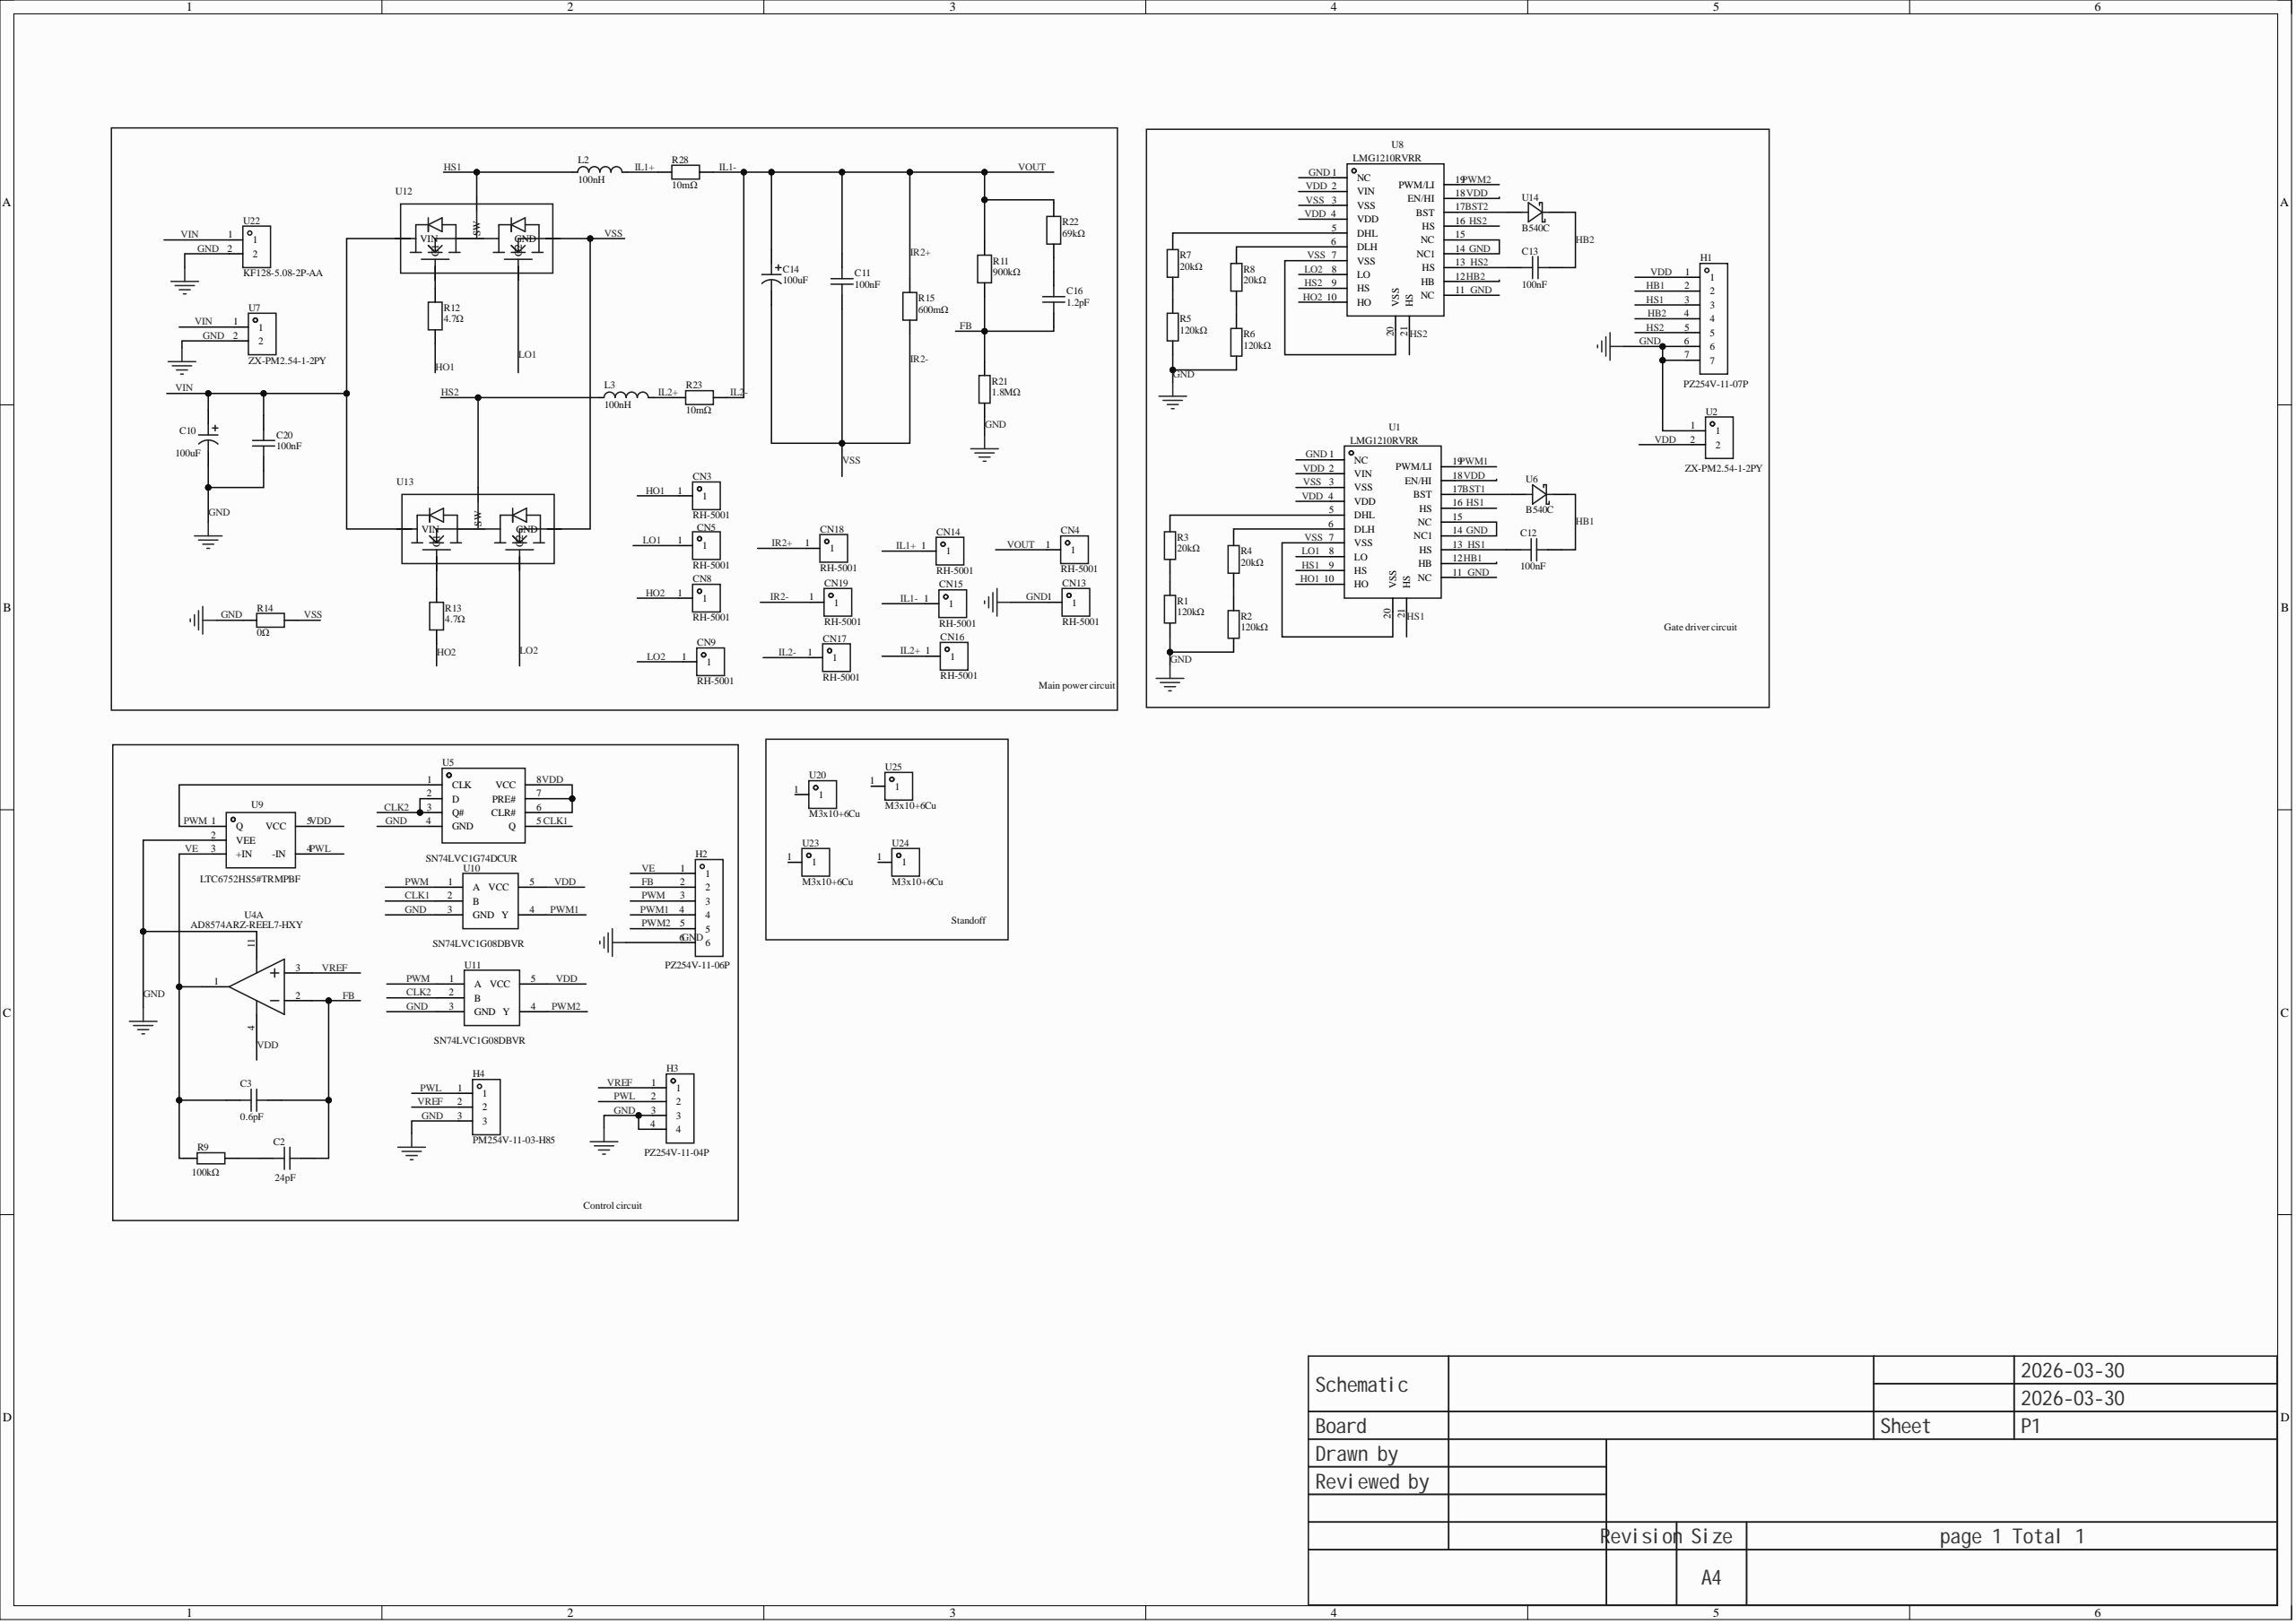Circuit board | Altium Designer | 63 parts | 38 nets
Bill of materials:
Comment,Description,Designator,Footprint,LibRef,Quantity
"24pF","Capacitance: 24pF; tolerance: ±1%; rated voltage: 50V; temperature coefficient: NP0;","C2","C0805","CC0805FRNPO9BN240","1"
"0.6pF","Capacitance: 0.6pF; rated voltage: 50V; temperature coefficient: C0G;","C3","C0603","GRM1885C1HR60WA01D","1"
"100uF","Capacitance: 100uF; tolerance: ±20%; rated voltage: 50V; ripple current: 140mA@120Hz;","C10","CAP-SMD_BD6.3-L6.6-W6.6-LS7.3-FD-H7.7","JVJ50V100M6x8","1"
"100nF","Capacitance: 100nF; tolerance: ±10%; rated voltage: 50V; temperature coefficient: X7R;","C11, C12, C13, C20","CAP-SMD_L2.0-W1.25","FCC0805B104K500DT","4"
"100uF","Capacitance: 100uF; tolerance: ±20%; rated voltage: 35V; ripple current: 2.9A@100kHz; equivalent series resistance (ESR): 30mΩ@100kHz; type: polymer;","C14","CAP-SMD_BD6.3-L6.6-W6.6-RD","MA35V100M6X8","1"
"1.2pF","Capacitance: 1.2pF; rated voltage: 250V; temperature coefficient: -;","C16","C0805","MCA08HQ1R2C251T7","1"
"RH-5001","Test pin, high-temperature nylon / phosphor bronze silver-plated, 5001 test point, 100x80mm","CN3, CN4, CN5, CN8, CN9, CN13, CN14, CN15, CN16, CN17, CN18, CN19","TEST-TH_BD2.54-P1.4_BLACK","RH-5001","12"
"PZ254V-11-07P","","H1","HDR-TH_7P-P2.54-V-M","PZ254V-11-07P","1"
"PZ254V-11-06P","","H2","HDR-TH_6P-P2.54-V-M","PZ254V-11-06P","1"
"PZ254V-11-04P","","H3","HDR-TH_4P-P2.54-V-M","PZ254V-11-04P","1"
"PM254V-11-03-H85","","H4","HDR-TH_3P-P2.54-V-F","PM254V-11-03-H85","1"
"100nH","Inductance: 100nH; tolerance: ±5%; rated current: 400mA; DC resistance (DCR): 460mΩ;","L2, L3","IND-SMD_L2.3-W1.8","AHW2012C-R10JTF","2"
"120kΩ","Resistor type: thick film resistor; resistance: 120kΩ; tolerance: ±1%; power: 125mW; working voltage: 150V; temperature coefficient: ±100ppm/?;","R1, R2, R5, R6","R0805","0805W8F1203T5E","4"
"20kΩ","Resistor type: thick film resistor; resistance: 20kΩ; tolerance: ±1%; power: 125mW; maximum working voltage: 150V; temperature coefficient: ±100ppm/?;","R3, R4, R7, R8","R0805","0805W8F2002T5E","4"
"100kΩ","Resistor type: thick film resistor; resistance: 100kΩ; tolerance: ±1%; power: 125mW; working voltage: 150V; temperature coefficient: ±100ppm/?;","R9","R0805","0805W8F1003T5E","1"
"900kΩ","Resistor type: thin film resistor; resistance: 900kΩ; tolerance: ±0.1%; power: 250mW; temperature coefficient: ±50ppm/?;","R11","R1206","RT1206BRE07900KL","1"
"4.7Ω","Resistor type: thick film resistor; resistance: 4.7Ω; tolerance: ±5%; power: 125mW; working voltage: 150V; temperature coefficient: ±200ppm/?;","R12, R13","R0805","FRC0805J4R7 TS","2"
"0Ω","Resistor type: sampling resistor; alloy resistor; resistance: 0Ω; tolerance: ±1%; power: 1W; mounting: SMD;","R14","R1206","RE1206F1R000","1"
"600mΩ","Resistor type: thick film resistor; resistance: 600mΩ; tolerance: ±1%; power: 250mW; working voltage: 500V; temperature coefficient: ±200ppm/?;","R15","R1206","FRL1206FR600TS","1"
"1.8MΩ","Resistor type: thick film resistor; resistance: 1.8MΩ; tolerance: ±1%; power: 125mW; working voltage: 150V; temperature coefficient: ±100ppm/?;","R21","R0805","0805W8F1804T5E","1"
"69kΩ","Resistor type: thin film resistor; resistance: 69kΩ; tolerance: ±0.1%; power: 100mW; temperature coefficient: ±25ppm/?;","R22","R0603","RT0603BRD0769KL","1"
"10mΩ","Resistor type: alloy resistor; resistance: 10mΩ; tolerance: ±1%; power: 750mW; temperature coefficient: ±50ppm/?; mounting: SMD;","R23, R28","R0805","RE0805FBR010","2"
"LMG1210RVRR","Driver configuration: half-bridge; load type: MOSFET; driver channels: 2; sink current (IOL): 3A; source current (IOH): 1.5A; working voltage: 6V~18V; rise time (tr): 500ps; fall time (tf): 2.3ns;","U1, U8","WQFN-19_L4.0-W3.0-P0.50-BL-EP_LMG1210RVRR","LMG1210RVRR","2"
"ZX-PM2.54-1-2PY","","U2, U7","HDR-TH_2P-P2.54-V-F","ZX-PM2.54-1-2PY","2"
"AD8574ARZ-REEL7-HXY","Amplifier count: quad; gain-bandwidth product (GBP): 1.5MHz; input bias current (Ib): 70pA; input offset voltage (Vos): 2uV; slew rate (SR): 1.2V/us; rail-to-rail: rail-to-rail input, rail-to-rail output;","U4","SOP-14_L8.7-W3.9-P1.27-LS6.0-BL","AD8574ARZ-REEL7-HXY","1"
"SN74LVC1G74DCUR","Type: D-type; working voltage: 1.65V~5.5V; clock frequency (fc): 200MHz; number of elements: 1; bits per element: 1; propagation delay (tpd): 6.4ns@5V,50pF; quiescent current (Iq): 10uA;","U5","SSOP-8_L2.0-W2.3-P0.50-LS3.1-BR","SN74LVC1G74DCUR","1"
"B540C","Diode configuration: single; forward voltage (Vf): 550mV@5A; DC reverse voltage (Vr): 40V; rectifier current: 5A;","U6, U14","SMC_L6.9-W5.9-LS7.9-RD","B540C_C6807783","2"
"LTC6752HS5#TRMPBF","Comparator count: single; input offset voltage (Vos): 1.2mV; input bias current (Ib): 1.35uA; rail-to-rail: rail-to-rail input;","U9","SOT-23-5_L3.0-W1.7-P0.95-LS2.8-BL","LTC6752HS5#TRMPBF","1"
"SN74LVC1G08DBVR","Logic type: AND gate; channels: 1; working voltage: 1.65V~5.5V; quiescent current (Iq): 10uA; propagation delay (tpd): 4ns@5V,50pF;","U10, U11","SOT-23-5_L3.0-W1.7-P0.95-LS2.8-BR","SN74LVC1G08DBVR","2"
"","","U12, U13","2111","EPC2111","2"
"M3x10+6Cu","M3x10+6","U20, U23, U24, U25","SMD_L4.7-W4.7-D3.0","M3x10+6Cu","4"
"KF128-5.08-2P-AA","","U22","CONN-TH_P5.08_KF128-5.08-2P","KF128-5.08-2P-AA","1"
Netlist (Protel format):
[
C2
C0805
24pF



]
[
C3
C0603
0.6pF



]
[
C10
CAP-SMD_BD6.3-L6.6-W6.6-LS7.3-FD-H7.7
100uF



]
[
C11
CAP-SMD_L2.0-W1.25
100nF



]
[
C12
CAP-SMD_L2.0-W1.25
100nF



]
[
C13
CAP-SMD_L2.0-W1.25
100nF



]
[
C14
CAP-SMD_BD6.3-L6.6-W6.6-RD
100uF



]
[
C16
C0805
1.2pF



]
[
C20
CAP-SMD_L2.0-W1.25
100nF



]
[
CN3
TEST-TH_BD2.54-P1.4_BLACK
RH-5001



]
[
CN4
TEST-TH_BD2.54-P1.4_BLACK
RH-5001



]
[
CN5
TEST-TH_BD2.54-P1.4_BLACK
RH-5001



]
[
CN8
TEST-TH_BD2.54-P1.4_BLACK
RH-5001



]
[
CN9
TEST-TH_BD2.54-P1.4_BLACK
RH-5001



]
[
CN13
TEST-TH_BD2.54-P1.4_BLACK
RH-5001



]
[
CN14
TEST-TH_BD2.54-P1.4_BLACK
RH-5001



]
[
CN15
TEST-TH_BD2.54-P1.4_BLACK
RH-5001



]
[
CN16
TEST-TH_BD2.54-P1.4_BLACK
RH-5001



]
[
CN17
TEST-TH_BD2.54-P1.4_BLACK
RH-5001



]
[
CN18
TEST-TH_BD2.54-P1.4_BLACK
RH-5001



]
[
CN19
TEST-TH_BD2.54-P1.4_BLACK
RH-5001



]
[
H1
HDR-TH_7P-P2.54-V-M
PZ254V-11-07P



]
[
H2
HDR-TH_6P-P2.54-V-M
PZ254V-11-06P



]
[
H3
HDR-TH_4P-P2.54-V-M
PZ254V-11-04P



]
[
H4
HDR-TH_3P-P2.54-V-F
PM254V-11-03-H85



]
[
L2
IND-SMD_L2.3-W1.8
100nH



]
[
L3
IND-SMD_L2.3-W1.8
100nH



]
[
R1
R0805
120kΩ



]
[
R2
R0805
120kΩ



]
[
R3
R0805
20kΩ



]
[
R4
R0805
20kΩ



]
[
R5
R0805
120kΩ



]
[
R6
R0805
120kΩ



]
[
R7
R0805
20kΩ



]
[
R8
R0805
20kΩ



]
[
R9
R0805
100kΩ



]
[
R11
R1206
900kΩ



]
[
R12
R0805
4.7Ω



]
[
R13
R0805
4.7Ω



]
[
R14
R1206
0Ω



]
[
R15
R1206
600mΩ



]
[
R21
R0805
1.8MΩ



]
[
R22
R0603
69kΩ



]
[
R23
R0805
10mΩ



]
[
R28
R0805
10mΩ



]
[
U1
WQFN-19_L4.0-W3.0-P0.50-BL-EP_LMG1210RVRR
LMG1210RVRR



]
[
U2
HDR-TH_2P-P2.54-V-F
ZX-PM2.54-1-2PY



]
[
U4
SOP-14_L8.7-W3.9-P1.27-LS6.0-BL
AD8574ARZ-REEL7-HXY



]
[
U5
SSOP-8_L2.0-W2.3-P0.50-LS3.1-BR
SN74LVC1G74DCUR



]
[
U6
SMC_L6.9-W5.9-LS7.9-RD
B540C



]
[
U7
HDR-TH_2P-P2.54-V-F
ZX-PM2.54-1-2PY



]
[
U8
WQFN-19_L4.0-W3.0-P0.50-BL-EP_LMG1210RVRR
LMG1210RVRR



]
[
U9
SOT-23-5_L3.0-W1.7-P0.95-LS2.8-BL
LTC6752HS5#TRMPBF



]
[
U10
SOT-23-5_L3.0-W1.7-P0.95-LS2.8-BR
SN74LVC1G08DBVR



]
[
U11
SOT-23-5_L3.0-W1.7-P0.95-LS2.8-BR
SN74LVC1G08DBVR



]
[
U12
2111




]
[
U13
2111




]
[
U14
SMC_L6.9-W5.9-LS7.9-RD
B540C



]
[
U20
SMD_L4.7-W4.7-D3.0
M3x10+6Cu



]
[
U22
CONN-TH_P5.08_KF128-5.08-2P
KF128-5.08-2P-AA



]
[
U23
SMD_L4.7-W4.7-D3.0
M3x10+6Cu



]
[
U24
SMD_L4.7-W4.7-D3.0
M3x10+6Cu



]
[
U25
SMD_L4.7-W4.7-D3.0
M3x10+6Cu



]
(
VREF
H3-1
H4-2
U4-3
)
(
VIN
C10-1
C20-2
U7-1
U12-2
U13-2
U22-1
)
(
VE
C3-1
H2-1
R9-1
U4-1
U9-3
)
(
VDD
H1-1
U1-2
U1-4
U1-18
U2-2
U4-4
U5-6
U5-7
U5-8
U8-2
U8-4
U8-18
U9-5
U10-5
U11-5
)
(
PWM2
H2-5
U8-19
U11-4
)
(
PWM1
H2-4
U1-19
U10-4
)
(
PWM
H2-3
U5-1
U9-1
U10-1
U11-1
)
(
PWL
H3-2
H4-1
U9-4
)
(
NetR13_2
R13-2
U13-1
)
(
NetR12_2
R12-2
U12-1
)
(
NetR8_2
R8-2
U8-6
)
(
NetR7_2
R7-2
U8-5
)
(
NetR6_2
R6-2
R8-1
)
(
NetR5_2
R5-2
R7-1
)
(
NetR4_2
R4-2
U1-6
)
(
NetR3_2
R3-2
U1-5
)
(
NetR2_2
R2-2
R4-1
)
(
NetR1_2
R1-2
R3-1
)
(
NetC16_2
C16-2
R22-1
)
(
NetC2_1
C2-1
R9-2
)
(
LO2
CN9-1
U8-8
U13-3
)
(
LO1
CN5-1
U1-8
U12-3
)
(
IR2-
C11-1
C14-2
CN19-1
R14-2
R15-1
U1-3
U1-7
U1-20
U8-3
U8-7
U8-20
U12-4
U13-4
)
(
IL2+
CN16-1
L3-2
R23-1
)
(
IL1-
C11-2
C14-1
CN4-1
CN15-1
CN17-1
CN18-1
R11-2
R15-2
R22-2
R23-2
R28-2
)
(
IL1+
CN14-1
L2-2
R28-1
)
(
HS2
C13-1
H1-5
L3-1
U8-9
U8-13
U8-16
U8-21
U13-5
)
(
HS1
C12-1
H1-3
L2-1
U1-9
U1-13
U1-16
U1-21
U12-5
)
(
HO2
CN8-1
R13-1
U8-10
)
(
HO1
CN3-1
R12-1
U1-10
)
(
HB2
C13-2
H1-4
U8-12
U14-1
)
(
HB1
C12-2
H1-2
U1-12
U6-1
)
(
GND
C10-2
C20-1
CN13-1
H1-6
H1-7
H2-6
H3-3
H3-4
H4-3
R1-1
R2-1
R5-1
R6-1
R14-1
R21-1
U1-1
U1-11
U1-14
U1-15
U2-1
U4-11
U5-4
U7-2
U8-1
U8-11
U8-14
U8-15
U9-2
U10-3
U11-3
U22-2
)
(
FB
C2-2
C3-2
C16-1
H2-2
R11-1
R21-2
U4-2
)
(
CLK2
U5-2
U5-3
U11-2
)
(
CLK1
U5-5
U10-2
)
(
BST2
U8-17
U14-2
)
(
BST1
U1-17
U6-2
)